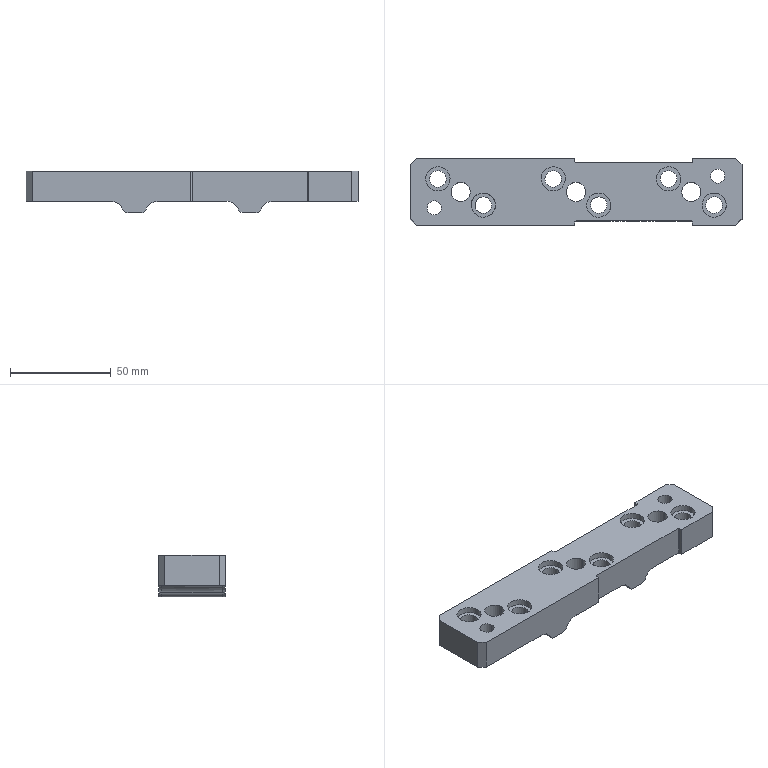Part | STEP file | 1_id1186_x_t | 1 solid | 98 faces | box 164.45 x 32.752 x 20.792 mm | volume 70018 mm3 | cylinder 60 | plane 30 | sphere 4 | torus 4 | commonest cylinder face diameters 12 x26 8.2 x12 9.52 x6 1 x4 5.85 x4 7 x4